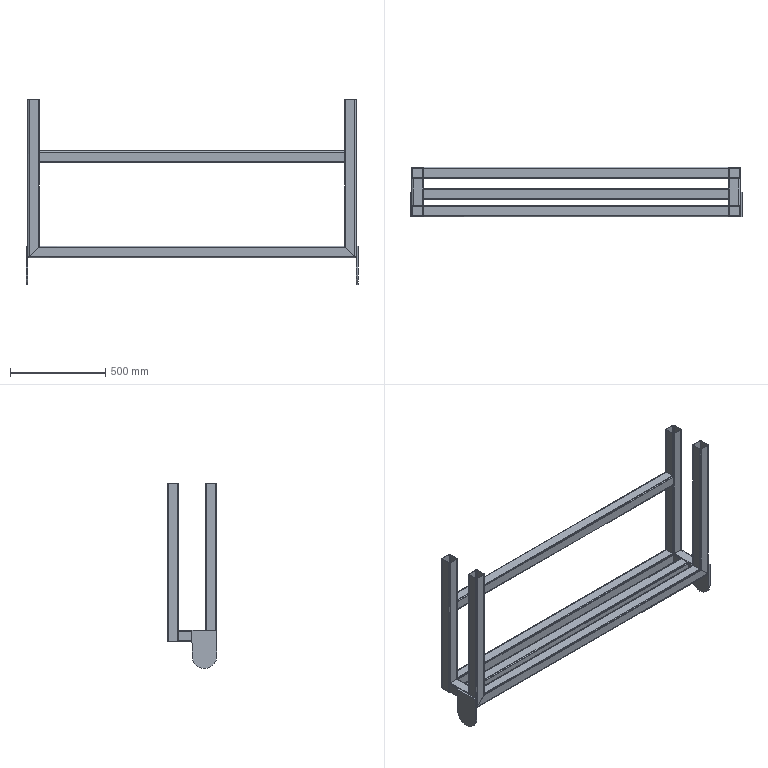Part | STEP file | Underframe_Default<Machined> | 12 solids | 194 faces | box 1740 x 260 x 970 mm | volume 7091962 mm3 | plane 110 | cylinder 84 | commonest cylinder face diameters 6 x40 12 x40 130 x4